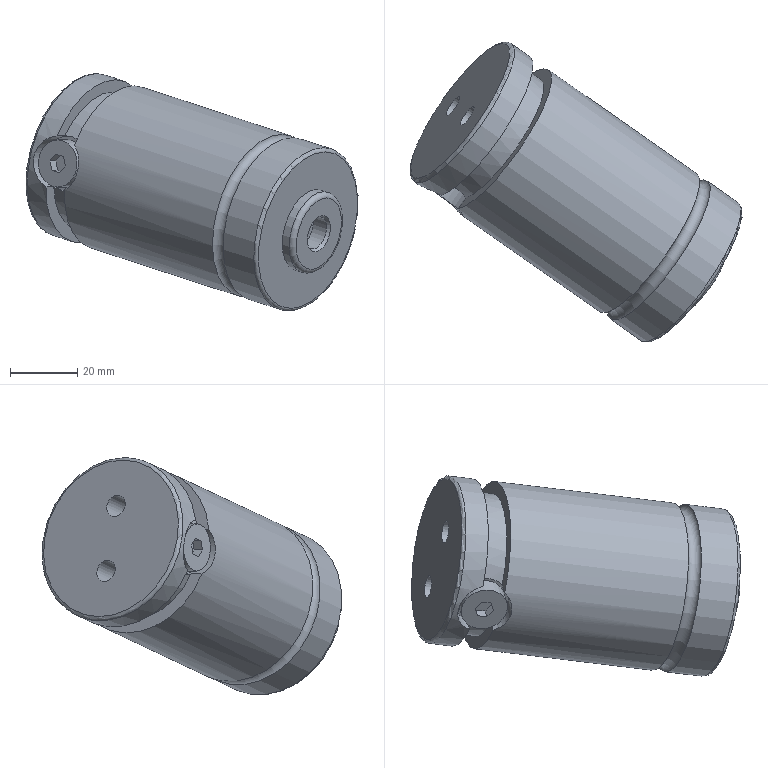Part | NX | features solid 2 | 1 solid | 38 faces | box 98.809 x 89.274 x 70.583 mm | volume 167634 mm3 | plane 17 | cylinder 13 | torus 4 | cone 4 | commonest cylinder face diameters 6.6 x3 14 x3 50.2 x3 10 x1 16.4 x1 25 x1
STEP:
#1=CARTESIAN_POINT('',(-50.295,651.708,-483.98));
#2=VERTEX_POINT('',#1);
#3=CARTESIAN_POINT('',(-55.617,655.435,-508.225));
#4=DIRECTION('',(-0.7912,0.554,0.2588));
#5=DIRECTION('',(0.212,-0.1485,0.9659));
#6=AXIS2_PLACEMENT_3D('',#3,#4,#5);
#7=CIRCLE('',#6,25.1);
#8=EDGE_CURVE('',#2,#2,#7,.T.);
#9=ORIENTED_EDGE('',*,*,#8,.F.);
#10=EDGE_LOOP('',(#9));
#11=FACE_BOUND('',#10,.T.);
#12=CARTESIAN_POINT('',(-47.13,649.492,-485.016));
#13=VERTEX_POINT('',#12);
#14=CARTESIAN_POINT('',(-52.452,653.218,-509.26));
#15=DIRECTION('',(-0.7912,0.554,0.2588));
#16=DIRECTION('',(0.212,-0.1485,0.9659));
#17=AXIS2_PLACEMENT_3D('',#14,#15,#16);
#18=CIRCLE('',#17,25.1);
#19=EDGE_CURVE('',#13,#13,#18,.T.);
#20=ORIENTED_EDGE('',*,*,#19,.T.);
#21=EDGE_LOOP('',(#20));
#22=FACE_BOUND('',#21,.T.);
#23=CARTESIAN_POINT('',(-54.034,654.327,-508.743));
#24=DIRECTION('',(0.7912,-0.554,-0.2588));
#25=DIRECTION('',(-0.5736,-0.8192,0.));
#26=AXIS2_PLACEMENT_3D('',#23,#24,#25);
#27=TOROIDAL_SURFACE('',#26,25.1,2.);
#28=ADVANCED_FACE('',(#11,#22),#27,.F.);
#29=CARTESIAN_POINT('',(-38.031,643.121,-487.992));
#30=VERTEX_POINT('',#29);
#31=CARTESIAN_POINT('',(-43.353,646.847,-512.237));
#32=DIRECTION('',(-0.7912,0.554,0.2588));
#33=DIRECTION('',(0.212,-0.1485,0.9659));
#34=AXIS2_PLACEMENT_3D('',#31,#32,#33);
#35=CIRCLE('',#34,25.1);
#36=EDGE_CURVE('',#30,#30,#35,.T.);
#37=ORIENTED_EDGE('',*,*,#36,.F.);
#38=EDGE_LOOP('',(#37));
#39=FACE_BOUND('',#38,.T.);
#40=CARTESIAN_POINT('',(-37.452,642.715,-489.217));
#41=VERTEX_POINT('',#40);
#42=CARTESIAN_POINT('',(-42.562,646.293,-512.495));
#43=DIRECTION('',(-0.7912,0.554,0.2588));
#44=DIRECTION('',(0.212,-0.1485,0.9659));
#45=AXIS2_PLACEMENT_3D('',#42,#43,#44);
#46=CIRCLE('',#45,24.1);
#47=EDGE_CURVE('',#41,#41,#46,.T.);
#48=ORIENTED_EDGE('',*,*,#47,.T.);
#49=EDGE_LOOP('',(#48));
#50=FACE_BOUND('',#49,.T.);
#51=CARTESIAN_POINT('',(-43.353,646.847,-512.237));
#52=DIRECTION('',(0.7912,-0.554,-0.2588));
#53=DIRECTION('',(-0.5736,-0.8192,0.));
#54=AXIS2_PLACEMENT_3D('',#51,#52,#53);
#55=TOROIDAL_SURFACE('',#54,24.1,1.);
#56=ADVANCED_FACE('',(#39,#50),#55,.T.);
#57=ORIENTED_EDGE('',*,*,#19,.F.);
#58=EDGE_LOOP('',(#57));
#59=FACE_BOUND('',#58,.T.);
#60=ORIENTED_EDGE('',*,*,#36,.T.);
#61=EDGE_LOOP('',(#60));
#62=FACE_BOUND('',#61,.T.);
#63=CARTESIAN_POINT('',(-47.902,650.033,-510.748));
#64=DIRECTION('',(-0.7912,0.554,0.2588));
#65=DIRECTION('',(0.5736,0.8192,0.));
#66=AXIS2_PLACEMENT_3D('',#63,#64,#65);
#67=CYLINDRICAL_SURFACE('',#66,25.1);
#68=ADVANCED_FACE('',(#59,#62),#67,.T.);
#69=CARTESIAN_POINT('',(-109.724,668.701,-487.213));
#70=VERTEX_POINT('',#69);
#71=CARTESIAN_POINT('',(-112.63,670.737,-500.456));
#72=VERTEX_POINT('',#71);
#73=CARTESIAN_POINT('',(-99.61,686.239,-493.835));
#74=DIRECTION('',(-0.7912,0.554,0.2588));
#75=DIRECTION('',(0.212,-0.1485,0.9659));
#76=AXIS2_PLACEMENT_3D('',#73,#74,#75);
#77=CIRCLE('',#76,21.3);
#78=EDGE_CURVE('',#70,#72,#77,.T.);
#79=ORIENTED_EDGE('',*,*,#78,.T.);
#80=CARTESIAN_POINT('',(-118.171,675.044,-499.566));
#81=VERTEX_POINT('',#80);
#82=CARTESIAN_POINT('',(-118.171,675.044,-499.566));
#83=CARTESIAN_POINT('',(-116.313,674.102,-500.892));
#84=CARTESIAN_POINT('',(-114.258,672.429,-501.217));
#85=CARTESIAN_POINT('',(-112.63,670.737,-500.456));
#86=B_SPLINE_CURVE_WITH_KNOTS('',3,(#82,#83,#84,#85),.UNSPECIFIED.,.F.,.F.,(4,4),(0.,0.007303),.UNSPECIFIED.);
#87=EDGE_CURVE('',#81,#72,#86,.T.);
#88=ORIENTED_EDGE('',*,*,#87,.F.);
#89=CARTESIAN_POINT('',(-114.859,672.725,-484.479));
#90=VERTEX_POINT('',#89);
#91=CARTESIAN_POINT('',(-105.149,690.117,-492.023));
#92=DIRECTION('',(-0.7912,0.554,0.2588));
#93=DIRECTION('',(0.212,-0.1485,0.9659));
#94=AXIS2_PLACEMENT_3D('',#91,#92,#93);
#95=CIRCLE('',#94,21.3);
#96=EDGE_CURVE('',#90,#81,#95,.T.);
#97=ORIENTED_EDGE('',*,*,#96,.F.);
#98=CARTESIAN_POINT('',(-109.724,668.701,-487.213));
#99=CARTESIAN_POINT('',(-110.787,669.998,-485.402));
#100=CARTESIAN_POINT('',(-112.684,671.561,-484.362));
#101=CARTESIAN_POINT('',(-114.859,672.725,-484.479));
#102=B_SPLINE_CURVE_WITH_KNOTS('',3,(#98,#99,#100,#101),.UNSPECIFIED.,.F.,.F.,(4,4),(0.,0.007305),.UNSPECIFIED.);
#103=EDGE_CURVE('',#70,#90,#102,.T.);
#104=ORIENTED_EDGE('',*,*,#103,.F.);
#105=EDGE_LOOP('',(#79,#88,#97,#104));
#106=FACE_BOUND('',#105,.T.);
#107=CARTESIAN_POINT('',(-102.379,688.178,-492.929));
#108=DIRECTION('',(-0.7912,0.554,0.2588));
#109=DIRECTION('',(0.5736,0.8192,0.));
#110=AXIS2_PLACEMENT_3D('',#107,#108,#109);
#111=CYLINDRICAL_SURFACE('',#110,21.3);
#112=ADVANCED_FACE('',(#106),#111,.T.);
#113=CARTESIAN_POINT('',(-105.366,690.269,-465.966));
#114=VERTEX_POINT('',#113);
#115=CARTESIAN_POINT('',(-110.687,693.995,-490.211));
#116=DIRECTION('',(-0.7912,0.554,0.2588));
#117=DIRECTION('',(0.212,-0.1485,0.9659));
#118=AXIS2_PLACEMENT_3D('',#115,#116,#117);
#119=CIRCLE('',#118,25.1);
#120=EDGE_CURVE('',#114,#114,#119,.T.);
#121=ORIENTED_EDGE('',*,*,#120,.F.);
#122=EDGE_LOOP('',(#121));
#123=FACE_BOUND('',#122,.T.);
#124=CARTESIAN_POINT('',(-117.175,669.417,-484.479));
#125=VERTEX_POINT('',#124);
#126=CARTESIAN_POINT('',(-120.487,671.736,-499.566));
#127=VERTEX_POINT('',#126);
#128=CARTESIAN_POINT('',(-105.149,690.117,-492.023));
#129=DIRECTION('',(-0.7912,0.554,0.2588));
#130=DIRECTION('',(0.212,-0.1485,0.9659));
#131=AXIS2_PLACEMENT_3D('',#128,#129,#130);
#132=CIRCLE('',#131,25.1);
#133=EDGE_CURVE('',#125,#127,#132,.T.);
#134=ORIENTED_EDGE('',*,*,#133,.T.);
#135=CARTESIAN_POINT('',(-117.175,669.417,-484.479));
#136=CARTESIAN_POINT('',(-118.703,670.274,-484.563));
#137=CARTESIAN_POINT('',(-121.8,671.637,-485.825));
#138=CARTESIAN_POINT('',(-124.63,672.867,-490.401));
#139=CARTESIAN_POINT('',(-124.012,673.182,-495.851));
#140=CARTESIAN_POINT('',(-121.788,672.435,-498.623));
#141=CARTESIAN_POINT('',(-120.487,671.736,-499.566));
#142=B_SPLINE_CURVE_WITH_KNOTS('',3,(#135,#136,#137,#138,#139,#140,#141),.UNSPECIFIED.,.F.,.F.,(4,1,1,1,4),(-0.01037,-0.005185,-0.000001062,0.005183,0.01037),.UNSPECIFIED.);
#143=EDGE_CURVE('',#125,#127,#142,.T.);
#144=ORIENTED_EDGE('',*,*,#143,.F.);
#145=EDGE_LOOP('',(#134,#144));
#146=FACE_BOUND('',#145,.T.);
#147=CARTESIAN_POINT('',(-107.918,692.056,-491.117));
#148=DIRECTION('',(-0.7912,0.554,0.2588));
#149=DIRECTION('',(0.5736,0.8192,0.));
#150=AXIS2_PLACEMENT_3D('',#147,#148,#149);
#151=CYLINDRICAL_SURFACE('',#150,25.1);
#152=ADVANCED_FACE('',(#123,#146),#151,.T.);
#153=CARTESIAN_POINT('',(-106.369,690.972,-466.674));
#154=VERTEX_POINT('',#153);
#155=CARTESIAN_POINT('',(-111.479,694.549,-489.952));
#156=DIRECTION('',(-0.7912,0.554,0.2588));
#157=DIRECTION('',(0.212,-0.1485,0.9659));
#158=AXIS2_PLACEMENT_3D('',#155,#156,#157);
#159=CIRCLE('',#158,24.1);
#160=EDGE_CURVE('',#154,#154,#159,.T.);
#161=ORIENTED_EDGE('',*,*,#160,.F.);
#162=EDGE_LOOP('',(#161));
#163=FACE_BOUND('',#162,.T.);
#164=ORIENTED_EDGE('',*,*,#120,.T.);
#165=EDGE_LOOP('',(#164));
#166=FACE_BOUND('',#165,.T.);
#167=CARTESIAN_POINT('',(-110.687,693.995,-490.211));
#168=DIRECTION('',(0.7912,-0.554,-0.2588));
#169=DIRECTION('',(-0.5736,-0.8192,0.));
#170=AXIS2_PLACEMENT_3D('',#167,#168,#169);
#171=TOROIDAL_SURFACE('',#170,24.1,1.);
#172=ADVANCED_FACE('',(#163,#166),#171,.T.);
#173=CARTESIAN_POINT('',(-37.854,642.997,-501.094));
#174=VERTEX_POINT('',#173);
#175=CARTESIAN_POINT('',(-40.504,644.853,-513.168));
#176=DIRECTION('',(-0.7912,0.554,0.2588));
#177=DIRECTION('',(0.212,-0.1485,0.9659));
#178=AXIS2_PLACEMENT_3D('',#175,#176,#177);
#179=CIRCLE('',#178,12.5);
#180=EDGE_CURVE('',#174,#174,#179,.T.);
#181=ORIENTED_EDGE('',*,*,#180,.F.);
#182=EDGE_LOOP('',(#181));
#183=FACE_BOUND('',#182,.T.);
#184=CARTESIAN_POINT('',(-36.985,642.389,-502.931));
#185=VERTEX_POINT('',#184);
#186=CARTESIAN_POINT('',(-39.317,644.022,-513.557));
#187=DIRECTION('',(-0.7912,0.554,0.2588));
#188=DIRECTION('',(0.212,-0.1485,0.9659));
#189=AXIS2_PLACEMENT_3D('',#186,#187,#188);
#190=CIRCLE('',#189,11.);
#191=EDGE_CURVE('',#185,#185,#190,.T.);
#192=ORIENTED_EDGE('',*,*,#191,.T.);
#193=EDGE_LOOP('',(#192));
#194=FACE_BOUND('',#193,.T.);
#195=CARTESIAN_POINT('',(-40.504,644.853,-513.168));
#196=DIRECTION('',(0.7912,-0.554,-0.2588));
#197=DIRECTION('',(-0.5736,-0.8192,0.));
#198=AXIS2_PLACEMENT_3D('',#195,#196,#197);
#199=TOROIDAL_SURFACE('',#198,11.,1.5);
#200=ADVANCED_FACE('',(#183,#194),#199,.T.);
#201=CARTESIAN_POINT('',(-39.911,644.437,-500.421));
#202=VERTEX_POINT('',#201);
#203=CARTESIAN_POINT('',(-42.562,646.293,-512.495));
#204=DIRECTION('',(0.7912,-0.554,-0.2588));
#205=DIRECTION('',(0.212,-0.1485,0.9659));
#206=AXIS2_PLACEMENT_3D('',#203,#204,#205);
#207=CIRCLE('',#206,12.5);
#208=EDGE_CURVE('',#202,#202,#207,.T.);
#209=ORIENTED_EDGE('',*,*,#208,.T.);
#210=EDGE_LOOP('',(#209));
#211=FACE_BOUND('',#210,.T.);
#212=ORIENTED_EDGE('',*,*,#180,.T.);
#213=EDGE_LOOP('',(#212));
#214=FACE_BOUND('',#213,.T.);
#215=CARTESIAN_POINT('',(-41.533,645.573,-512.832));
#216=DIRECTION('',(-0.7912,0.554,0.2588));
#217=DIRECTION('',(0.5736,0.8192,0.));
#218=AXIS2_PLACEMENT_3D('',#215,#216,#217);
#219=CYLINDRICAL_SURFACE('',#218,12.5);
#220=ADVANCED_FACE('',(#211,#214),#219,.T.);
#221=CARTESIAN_POINT('',(-100.146,686.614,-486.723));
#222=VERTEX_POINT('',#221);
#223=CARTESIAN_POINT('',(-103.354,688.86,-485.674));
#224=VERTEX_POINT('',#223);
#225=CARTESIAN_POINT('',(-101.75,687.737,-486.198));
#226=DIRECTION('',(-0.7912,0.554,0.2588));
#227=VECTOR('',#226,1000.);
#228=LINE('',#225,#227);
#229=EDGE_CURVE('',#222,#224,#228,.T.);
#230=ORIENTED_EDGE('',*,*,#229,.F.);
#231=CARTESIAN_POINT('',(-103.354,688.86,-485.674));
#232=CARTESIAN_POINT('',(-103.619,688.482,-485.674));
#233=CARTESIAN_POINT('',(-103.485,687.466,-485.647));
#234=CARTESIAN_POINT('',(-102.511,686.497,-485.862));
#235=CARTESIAN_POINT('',(-101.327,685.953,-486.352));
#236=CARTESIAN_POINT('',(-100.411,686.236,-486.723));
#237=CARTESIAN_POINT('',(-100.146,686.614,-486.723));
#238=B_SPLINE_CURVE_WITH_KNOTS('',3,(#231,#232,#233,#234,#235,#236,#237),.UNSPECIFIED.,.F.,.F.,(4,1,1,1,4),(0.,0.001359,0.002718,0.004077,0.005435),.UNSPECIFIED.);
#239=EDGE_CURVE('',#224,#222,#238,.T.);
#240=ORIENTED_EDGE('',*,*,#239,.F.);
#241=EDGE_LOOP('',(#230,#240));
#242=FACE_BOUND('',#241,.T.);
#243=CARTESIAN_POINT('',(-110.058,693.555,-483.481));
#244=VERTEX_POINT('',#243);
#245=CARTESIAN_POINT('',(-109.358,693.065,-480.293));
#246=DIRECTION('',(-0.7912,0.554,0.2588));
#247=DIRECTION('',(-0.212,0.1485,-0.9659));
#248=AXIS2_PLACEMENT_3D('',#245,#246,#247);
#249=CIRCLE('',#248,3.3);
#250=EDGE_CURVE('',#244,#244,#249,.T.);
#251=ORIENTED_EDGE('',*,*,#250,.T.);
#252=EDGE_LOOP('',(#251));
#253=FACE_BOUND('',#252,.T.);
#254=CARTESIAN_POINT('',(-96.211,683.859,-488.01));
#255=VERTEX_POINT('',#254);
#256=CARTESIAN_POINT('',(-95.512,683.369,-484.822));
#257=DIRECTION('',(0.7912,-0.554,-0.2588));
#258=DIRECTION('',(-0.212,0.1485,-0.9659));
#259=AXIS2_PLACEMENT_3D('',#256,#257,#258);
#260=CIRCLE('',#259,3.3);
#261=EDGE_CURVE('',#255,#255,#260,.T.);
#262=ORIENTED_EDGE('',*,*,#261,.T.);
#263=EDGE_LOOP('',(#262));
#264=FACE_BOUND('',#263,.T.);
#265=CARTESIAN_POINT('',(-102.435,688.217,-482.558));
#266=DIRECTION('',(0.7912,-0.554,-0.2588));
#267=DIRECTION('',(-0.5736,-0.8192,0.));
#268=AXIS2_PLACEMENT_3D('',#265,#266,#267);
#269=CYLINDRICAL_SURFACE('',#268,3.3);
#270=ADVANCED_FACE('',(#242,#253,#264),#269,.F.);
#271=ORIENTED_EDGE('',*,*,#261,.F.);
#272=EDGE_LOOP('',(#271));
#273=FACE_BOUND('',#272,.T.);
#274=CARTESIAN_POINT('',(-102.633,688.355,-482.493));
#275=VERTEX_POINT('',#274);
#276=VERTEX_LOOP('',#275);
#277=FACE_BOUND('',#276,.T.);
#278=CARTESIAN_POINT('',(-99.072,685.862,-483.658));
#279=DIRECTION('',(0.7912,-0.554,-0.2588));
#280=DIRECTION('',(-0.5736,-0.8192,0.));
#281=AXIS2_PLACEMENT_3D('',#278,#279,#280);
#282=CONICAL_SURFACE('',#281,1.65,0.3514);
#283=ADVANCED_FACE('',(#273,#277),#282,.T.);
#284=CARTESIAN_POINT('',(-106.873,691.325,-501.812));
#285=VERTEX_POINT('',#284);
#286=VERTEX_LOOP('',#285);
#287=FACE_BOUND('',#286,.T.);
#288=CARTESIAN_POINT('',(-99.052,685.848,-500.953));
#289=VERTEX_POINT('',#288);
#290=CARTESIAN_POINT('',(-99.752,686.338,-504.141));
#291=DIRECTION('',(-0.7912,0.554,0.2588));
#292=DIRECTION('',(0.212,-0.1485,0.9659));
#293=AXIS2_PLACEMENT_3D('',#290,#291,#292);
#294=CIRCLE('',#293,3.3);
#295=EDGE_CURVE('',#289,#289,#294,.T.);
#296=ORIENTED_EDGE('',*,*,#295,.T.);
#297=EDGE_LOOP('',(#296));
#298=FACE_BOUND('',#297,.T.);
#299=CARTESIAN_POINT('',(-103.313,688.831,-502.976));
#300=DIRECTION('',(0.7912,-0.554,-0.2588));
#301=DIRECTION('',(-0.5736,-0.8192,0.));
#302=AXIS2_PLACEMENT_3D('',#299,#300,#301);
#303=CONICAL_SURFACE('',#302,1.65,0.3514);
#304=ADVANCED_FACE('',(#287,#298),#303,.T.);
#305=CARTESIAN_POINT('',(-106.195,690.85,-498.617));
#306=VERTEX_POINT('',#305);
#307=CARTESIAN_POINT('',(-102.987,688.603,-499.666));
#308=VERTEX_POINT('',#307);
#309=CARTESIAN_POINT('',(-104.591,689.727,-499.142));
#310=DIRECTION('',(0.7912,-0.554,-0.2588));
#311=VECTOR('',#310,1000.);
#312=LINE('',#309,#311);
#313=EDGE_CURVE('',#306,#308,#312,.T.);
#314=ORIENTED_EDGE('',*,*,#313,.F.);
#315=CARTESIAN_POINT('',(-102.987,688.603,-499.666));
#316=CARTESIAN_POINT('',(-103.252,688.225,-499.666));
#317=CARTESIAN_POINT('',(-104.252,688.003,-499.693));
#318=CARTESIAN_POINT('',(-105.497,688.587,-499.478));
#319=CARTESIAN_POINT('',(-106.413,689.514,-498.987));
#320=CARTESIAN_POINT('',(-106.46,690.472,-498.617));
#321=CARTESIAN_POINT('',(-106.195,690.85,-498.617));
#322=B_SPLINE_CURVE_WITH_KNOTS('',3,(#315,#316,#317,#318,#319,#320,#321),.UNSPECIFIED.,.F.,.F.,(4,1,1,1,4),(0.,0.001359,0.002718,0.004077,0.005435),.UNSPECIFIED.);
#323=EDGE_CURVE('',#308,#306,#322,.T.);
#324=ORIENTED_EDGE('',*,*,#323,.F.);
#325=EDGE_LOOP('',(#314,#324));
#326=FACE_BOUND('',#325,.T.);
#327=ORIENTED_EDGE('',*,*,#295,.F.);
#328=EDGE_LOOP('',(#327));
#329=FACE_BOUND('',#328,.T.);
#330=CARTESIAN_POINT('',(-112.899,695.544,-496.424));
#331=VERTEX_POINT('',#330);
#332=CARTESIAN_POINT('',(-113.599,696.034,-499.612));
#333=DIRECTION('',(-0.7912,0.554,0.2588));
#334=DIRECTION('',(0.212,-0.1485,0.9659));
#335=AXIS2_PLACEMENT_3D('',#332,#333,#334);
#336=CIRCLE('',#335,3.3);
#337=EDGE_CURVE('',#331,#331,#336,.T.);
#338=ORIENTED_EDGE('',*,*,#337,.T.);
#339=EDGE_LOOP('',(#338));
#340=FACE_BOUND('',#339,.T.);
#341=CARTESIAN_POINT('',(-106.675,691.186,-501.876));
#342=DIRECTION('',(-0.7912,0.554,0.2588));
#343=DIRECTION('',(0.5736,0.8192,0.));
#344=AXIS2_PLACEMENT_3D('',#341,#342,#343);
#345=CYLINDRICAL_SURFACE('',#344,3.3);
#346=ADVANCED_FACE('',(#326,#329,#340),#345,.F.);
#347=CARTESIAN_POINT('',(-112.006,665.442,-487.213));
#348=VERTEX_POINT('',#347);
#349=CARTESIAN_POINT('',(-114.913,667.477,-500.456));
#350=VERTEX_POINT('',#349);
#351=CARTESIAN_POINT('',(-99.61,686.239,-493.835));
#352=DIRECTION('',(-0.7912,0.554,0.2588));
#353=DIRECTION('',(0.212,-0.1485,0.9659));
#354=AXIS2_PLACEMENT_3D('',#351,#352,#353);
#355=CIRCLE('',#354,25.1);
#356=EDGE_CURVE('',#348,#350,#355,.T.);
#357=ORIENTED_EDGE('',*,*,#356,.F.);
#358=CARTESIAN_POINT('',(-114.913,667.477,-500.456));
#359=CARTESIAN_POINT('',(-113.976,666.563,-500.029));
#360=CARTESIAN_POINT('',(-112.365,664.824,-498.559));
#361=CARTESIAN_POINT('',(-110.87,663.334,-494.883));
#362=CARTESIAN_POINT('',(-110.631,663.61,-490.663));
#363=CARTESIAN_POINT('',(-111.386,664.749,-488.229));
#364=CARTESIAN_POINT('',(-112.006,665.442,-487.213));
#365=B_SPLINE_CURVE_WITH_KNOTS('',3,(#358,#359,#360,#361,#362,#363,#364),.UNSPECIFIED.,.F.,.F.,(4,1,1,1,4),(-0.008143,-0.004072,-0.000000126,0.004071,0.008143),.UNSPECIFIED.);
#366=EDGE_CURVE('',#350,#348,#365,.T.);
#367=ORIENTED_EDGE('',*,*,#366,.F.);
#368=EDGE_LOOP('',(#357,#367));
#369=FACE_BOUND('',#368,.T.);
#370=ORIENTED_EDGE('',*,*,#8,.T.);
#371=EDGE_LOOP('',(#370));
#372=FACE_BOUND('',#371,.T.);
#373=CARTESIAN_POINT('',(-77.613,670.837,-501.03));
#374=DIRECTION('',(-0.7912,0.554,0.2588));
#375=DIRECTION('',(0.5736,0.8192,0.));
#376=AXIS2_PLACEMENT_3D('',#373,#374,#375);
#377=CYLINDRICAL_SURFACE('',#376,25.1);
#378=ADVANCED_FACE('',(#369,#372),#377,.T.);
#379=CARTESIAN_POINT('',(-112.387,671.869,-484.749));
#380=VERTEX_POINT('',#379);
#381=CARTESIAN_POINT('',(-114.126,673.086,-492.67));
#382=DIRECTION('',(0.5736,0.8192,0.));
#383=DIRECTION('',(0.212,-0.1485,0.9659));
#384=AXIS2_PLACEMENT_3D('',#381,#382,#383);
#385=CIRCLE('',#384,8.2);
#386=EDGE_CURVE('',#380,#380,#385,.T.);
#387=ORIENTED_EDGE('',*,*,#386,.T.);
#388=EDGE_LOOP('',(#387));
#389=FACE_BOUND('',#388,.T.);
#390=ORIENTED_EDGE('',*,*,#103,.T.);
#391=CARTESIAN_POINT('',(-116.169,670.854,-484.479));
#392=DIRECTION('',(-0.5736,-0.8192,0.));
#393=VECTOR('',#392,1000.);
#394=LINE('',#391,#393);
#395=EDGE_CURVE('',#90,#125,#394,.T.);
#396=ORIENTED_EDGE('',*,*,#395,.T.);
#397=ORIENTED_EDGE('',*,*,#143,.T.);
#398=CARTESIAN_POINT('',(-119.48,673.173,-499.566));
#399=DIRECTION('',(0.5736,0.8192,0.));
#400=VECTOR('',#399,1000.);
#401=LINE('',#398,#400);
#402=EDGE_CURVE('',#127,#81,#401,.T.);
#403=ORIENTED_EDGE('',*,*,#402,.T.);
#404=ORIENTED_EDGE('',*,*,#87,.T.);
#405=CARTESIAN_POINT('',(-113.739,669.153,-500.456));
#406=DIRECTION('',(-0.5736,-0.8192,0.));
#407=VECTOR('',#406,1000.);
#408=LINE('',#405,#407);
#409=EDGE_CURVE('',#72,#350,#408,.T.);
#410=ORIENTED_EDGE('',*,*,#409,.T.);
#411=ORIENTED_EDGE('',*,*,#366,.T.);
#412=CARTESIAN_POINT('',(-110.833,667.118,-487.213));
#413=DIRECTION('',(0.5736,0.8192,0.));
#414=VECTOR('',#413,1000.);
#415=LINE('',#412,#414);
#416=EDGE_CURVE('',#348,#70,#415,.T.);
#417=ORIENTED_EDGE('',*,*,#416,.T.);
#418=EDGE_LOOP('',(#390,#396,#397,#403,#404,#410,#411,#417));
#419=FACE_BOUND('',#418,.T.);
#420=CARTESIAN_POINT('',(-117.567,668.171,-492.67));
#421=DIRECTION('',(-0.5736,-0.8192,0.));
#422=DIRECTION('',(0.212,-0.1485,0.9659));
#423=AXIS2_PLACEMENT_3D('',#420,#421,#422);
#424=CYLINDRICAL_SURFACE('',#423,8.2);
#425=ADVANCED_FACE('',(#389,#419),#424,.F.);
#426=CARTESIAN_POINT('',(-112.642,672.047,-485.908));
#427=VERTEX_POINT('',#426);
#428=CARTESIAN_POINT('',(-114.126,673.086,-492.67));
#429=DIRECTION('',(-0.5736,-0.8192,0.));
#430=DIRECTION('',(0.212,-0.1485,0.9659));
#431=AXIS2_PLACEMENT_3D('',#428,#429,#430);
#432=CIRCLE('',#431,7.);
#433=EDGE_CURVE('',#427,#427,#432,.T.);
#434=ORIENTED_EDGE('',*,*,#433,.T.);
#435=EDGE_LOOP('',(#434));
#436=FACE_BOUND('',#435,.T.);
#437=CARTESIAN_POINT('',(-115.51,667.951,-485.908));
#438=VERTEX_POINT('',#437);
#439=CARTESIAN_POINT('',(-116.994,668.99,-492.67));
#440=DIRECTION('',(-0.5736,-0.8192,0.));
#441=DIRECTION('',(0.212,-0.1485,0.9659));
#442=AXIS2_PLACEMENT_3D('',#439,#440,#441);
#443=CIRCLE('',#442,7.);
#444=EDGE_CURVE('',#438,#438,#443,.T.);
#445=ORIENTED_EDGE('',*,*,#444,.F.);
#446=EDGE_LOOP('',(#445));
#447=FACE_BOUND('',#446,.T.);
#448=CARTESIAN_POINT('',(-103.17,688.732,-492.67));
#449=DIRECTION('',(0.5736,0.8192,0.));
#450=DIRECTION('',(-0.212,0.1485,-0.9659));
#451=AXIS2_PLACEMENT_3D('',#448,#449,#450);
#452=CYLINDRICAL_SURFACE('',#451,7.);
#453=ADVANCED_FACE('',(#436,#447),#452,.T.);
#454=CARTESIAN_POINT('',(-103.17,688.732,-492.67));
#455=DIRECTION('',(0.5736,0.8192,0.));
#456=DIRECTION('',(0.212,-0.1485,0.9659));
#457=AXIS2_PLACEMENT_3D('',#454,#455,#456);
#458=CIRCLE('',#457,7.);
#459=EDGE_CURVE('',#308,#306,#458,.T.);
#460=ORIENTED_EDGE('',*,*,#459,.F.);
#461=ORIENTED_EDGE('',*,*,#323,.T.);
#462=EDGE_LOOP('',(#460,#461));
#463=FACE_BOUND('',#462,.T.);
#464=CARTESIAN_POINT('',(-103.17,688.732,-492.67));
#465=DIRECTION('',(0.5736,0.8192,0.));
#466=DIRECTION('',(-0.212,0.1485,-0.9659));
#467=AXIS2_PLACEMENT_3D('',#464,#465,#466);
#468=CYLINDRICAL_SURFACE('',#467,7.);
#469=ADVANCED_FACE('',(#463),#468,.T.);
#470=ORIENTED_EDGE('',*,*,#239,.T.);
#471=CARTESIAN_POINT('',(-103.17,688.732,-492.67));
#472=DIRECTION('',(0.5736,0.8192,0.));
#473=DIRECTION('',(0.212,-0.1485,0.9659));
#474=AXIS2_PLACEMENT_3D('',#471,#472,#473);
#475=CIRCLE('',#474,7.);
#476=EDGE_CURVE('',#224,#222,#475,.T.);
#477=ORIENTED_EDGE('',*,*,#476,.F.);
#478=EDGE_LOOP('',(#470,#477));
#479=FACE_BOUND('',#478,.T.);
#480=CARTESIAN_POINT('',(-103.17,688.732,-492.67));
#481=DIRECTION('',(0.5736,0.8192,0.));
#482=DIRECTION('',(-0.212,0.1485,-0.9659));
#483=AXIS2_PLACEMENT_3D('',#480,#481,#482);
#484=CYLINDRICAL_SURFACE('',#483,7.);
#485=ADVANCED_FACE('',(#479),#484,.T.);
#486=CARTESIAN_POINT('',(-36.105,648.609,-513.557));
#487=VERTEX_POINT('',#486);
#488=CARTESIAN_POINT('',(-39.317,644.022,-513.557));
#489=DIRECTION('',(0.7912,-0.554,-0.2588));
#490=DIRECTION('',(0.5736,0.8192,0.));
#491=AXIS2_PLACEMENT_3D('',#488,#489,#490);
#492=CIRCLE('',#491,5.6);
#493=EDGE_CURVE('',#487,#487,#492,.T.);
#494=ORIENTED_EDGE('',*,*,#493,.T.);
#495=EDGE_LOOP('',(#494));
#496=FACE_BOUND('',#495,.T.);
#497=CARTESIAN_POINT('',(-37.241,648.671,-513.298));
#498=VERTEX_POINT('',#497);
#499=CARTESIAN_POINT('',(-40.109,644.576,-513.298));
#500=DIRECTION('',(-0.7912,0.554,0.2588));
#501=DIRECTION('',(0.5736,0.8192,0.));
#502=AXIS2_PLACEMENT_3D('',#499,#500,#501);
#503=CIRCLE('',#502,5.);
#504=EDGE_CURVE('',#498,#498,#503,.T.);
#505=ORIENTED_EDGE('',*,*,#504,.T.);
#506=EDGE_LOOP('',(#505));
#507=FACE_BOUND('',#506,.T.);
#508=CARTESIAN_POINT('',(-39.713,644.299,-513.427));
#509=DIRECTION('',(0.7912,-0.554,-0.2588));
#510=DIRECTION('',(-0.5736,-0.8192,0.));
#511=AXIS2_PLACEMENT_3D('',#508,#509,#510);
#512=CONICAL_SURFACE('',#511,5.3,0.5404);
#513=ADVANCED_FACE('',(#496,#507),#512,.F.);
#514=ORIENTED_EDGE('',*,*,#504,.F.);
#515=EDGE_LOOP('',(#514));
#516=FACE_BOUND('',#515,.T.);
#517=CARTESIAN_POINT('',(-41.197,651.441,-512.004));
#518=VERTEX_POINT('',#517);
#519=CARTESIAN_POINT('',(-44.065,647.346,-512.004));
#520=DIRECTION('',(-0.7912,0.554,0.2588));
#521=DIRECTION('',(0.5736,0.8192,0.));
#522=AXIS2_PLACEMENT_3D('',#519,#520,#521);
#523=CIRCLE('',#522,5.);
#524=EDGE_CURVE('',#518,#518,#523,.T.);
#525=ORIENTED_EDGE('',*,*,#524,.T.);
#526=EDGE_LOOP('',(#525));
#527=FACE_BOUND('',#526,.T.);
#528=CARTESIAN_POINT('',(-42.087,645.961,-512.651));
#529=DIRECTION('',(-0.7912,0.554,0.2588));
#530=DIRECTION('',(0.5736,0.8192,0.));
#531=AXIS2_PLACEMENT_3D('',#528,#529,#530);
#532=CYLINDRICAL_SURFACE('',#531,5.);
#533=ADVANCED_FACE('',(#516,#527),#532,.F.);
#534=CARTESIAN_POINT('',(-42.172,650.049,-512.004));
#535=VERTEX_POINT('',#534);
#536=CARTESIAN_POINT('',(-44.065,647.346,-512.004));
#537=DIRECTION('',(-0.7912,0.554,0.2588));
#538=DIRECTION('',(0.5736,0.8192,0.));
#539=AXIS2_PLACEMENT_3D('',#536,#537,#538);
#540=CIRCLE('',#539,3.3);
#541=EDGE_CURVE('',#535,#535,#540,.T.);
#542=ORIENTED_EDGE('',*,*,#541,.F.);
#543=EDGE_LOOP('',(#542));
#544=FACE_BOUND('',#543,.T.);
#545=CARTESIAN_POINT('',(-48.502,654.481,-509.933));
#546=VERTEX_POINT('',#545);
#547=CARTESIAN_POINT('',(-50.395,651.778,-509.933));
#548=DIRECTION('',(-0.7912,0.554,0.2588));
#549=DIRECTION('',(0.5736,0.8192,0.));
#550=AXIS2_PLACEMENT_3D('',#547,#548,#549);
#551=CIRCLE('',#550,3.3);
#552=EDGE_CURVE('',#546,#546,#551,.T.);
#553=ORIENTED_EDGE('',*,*,#552,.T.);
#554=EDGE_LOOP('',(#553));
#555=FACE_BOUND('',#554,.T.);
#556=CARTESIAN_POINT('',(-47.23,649.562,-510.968));
#557=DIRECTION('',(-0.7912,0.554,0.2588));
#558=DIRECTION('',(0.5736,0.8192,0.));
#559=AXIS2_PLACEMENT_3D('',#556,#557,#558);
#560=CYLINDRICAL_SURFACE('',#559,3.3);
#561=ADVANCED_FACE('',(#544,#555),#560,.F.);
#562=CARTESIAN_POINT('',(-51.977,652.886,-509.416));
#563=VERTEX_POINT('',#562);
#564=VERTEX_LOOP('',#563);
#565=FACE_BOUND('',#564,.T.);
#566=ORIENTED_EDGE('',*,*,#552,.F.);
#567=EDGE_LOOP('',(#566));
#568=FACE_BOUND('',#567,.T.);
#569=CARTESIAN_POINT('',(-51.186,652.332,-509.674));
#570=DIRECTION('',(0.7912,-0.554,-0.2588));
#571=DIRECTION('',(-0.5736,-0.8192,0.));
#572=AXIS2_PLACEMENT_3D('',#569,#570,#571);
#573=CONICAL_SURFACE('',#572,1.65,1.026);
#574=ADVANCED_FACE('',(#565,#568),#573,.F.);
#575=ORIENTED_EDGE('',*,*,#524,.F.);
#576=EDGE_LOOP('',(#575));
#577=FACE_BOUND('',#576,.T.);
#578=ORIENTED_EDGE('',*,*,#541,.T.);
#579=EDGE_LOOP('',(#578));
#580=FACE_BOUND('',#579,.T.);
#581=CARTESIAN_POINT('',(-41.685,650.745,-512.004));
#582=DIRECTION('',(-0.7912,0.554,0.2588));
#583=DIRECTION('',(0.5736,0.8192,0.));
#584=AXIS2_PLACEMENT_3D('',#581,#582,#583);
#585=PLANE('',#584);
#586=ADVANCED_FACE('',(#577,#580),#585,.F.);
#587=CARTESIAN_POINT('',(-114.71,667.391,-493.417));
#588=VERTEX_POINT('',#587);
#589=CARTESIAN_POINT('',(-115.322,667.82,-490.629));
#590=VERTEX_POINT('',#589);
#591=CARTESIAN_POINT('',(-115.725,668.102,-488.79));
#592=DIRECTION('',(-0.212,0.1485,0.9659));
#593=VECTOR('',#592,1000.);
#594=LINE('',#591,#593);
#595=EDGE_CURVE('',#588,#590,#594,.T.);
#596=ORIENTED_EDGE('',*,*,#595,.T.);
#597=CARTESIAN_POINT('',(-113.601,670.277,-490.629));
#598=VERTEX_POINT('',#597);
#599=CARTESIAN_POINT('',(-115.895,667.,-490.629));
#600=DIRECTION('',(0.5736,0.8192,0.));
#601=VECTOR('',#600,1000.);
#602=LINE('',#599,#601);
#603=EDGE_CURVE('',#590,#598,#602,.T.);
#604=ORIENTED_EDGE('',*,*,#603,.T.);
#605=CARTESIAN_POINT('',(-112.989,669.848,-493.417));
#606=VERTEX_POINT('',#605);
#607=CARTESIAN_POINT('',(-113.601,670.277,-490.629));
#608=DIRECTION('',(0.212,-0.1485,-0.9659));
#609=VECTOR('',#608,1000.);
#610=LINE('',#607,#609);
#611=EDGE_CURVE('',#598,#606,#610,.T.);
#612=ORIENTED_EDGE('',*,*,#611,.T.);
#613=CARTESIAN_POINT('',(-115.283,666.572,-493.417));
#614=DIRECTION('',(0.5736,0.8192,0.));
#615=VECTOR('',#614,1000.);
#616=LINE('',#613,#615);
#617=EDGE_CURVE('',#588,#606,#616,.T.);
#618=ORIENTED_EDGE('',*,*,#617,.F.);
#619=EDGE_LOOP('',(#596,#604,#612,#618));
#620=FACE_BOUND('',#619,.T.);
#621=CARTESIAN_POINT('',(-115.895,667.,-490.629));
#622=DIRECTION('',(0.7912,-0.554,0.2588));
#623=DIRECTION('',(0.212,-0.1485,-0.9659));
#624=AXIS2_PLACEMENT_3D('',#621,#622,#623);
#625=PLANE('',#624);
#626=ADVANCED_FACE('',(#620),#625,.F.);
#627=CARTESIAN_POINT('',(-117.606,669.419,-489.882));
#628=VERTEX_POINT('',#627);
#629=CARTESIAN_POINT('',(-121.189,671.928,-488.71));
#630=DIRECTION('',(-0.7912,0.554,0.2588));
#631=VECTOR('',#630,1000.);
#632=LINE('',#629,#631);
#633=EDGE_CURVE('',#590,#628,#632,.T.);
#634=ORIENTED_EDGE('',*,*,#633,.T.);
#635=CARTESIAN_POINT('',(-115.885,671.876,-489.882));
#636=VERTEX_POINT('',#635);
#637=CARTESIAN_POINT('',(-118.179,668.6,-489.882));
#638=DIRECTION('',(0.5736,0.8192,0.));
#639=VECTOR('',#638,1000.);
#640=LINE('',#637,#639);
#641=EDGE_CURVE('',#628,#636,#640,.T.);
#642=ORIENTED_EDGE('',*,*,#641,.T.);
#643=CARTESIAN_POINT('',(-115.885,671.876,-489.882));
#644=DIRECTION('',(0.7912,-0.554,-0.2588));
#645=VECTOR('',#644,1000.);
#646=LINE('',#643,#645);
#647=EDGE_CURVE('',#636,#598,#646,.T.);
#648=ORIENTED_EDGE('',*,*,#647,.T.);
#649=ORIENTED_EDGE('',*,*,#603,.F.);
#650=EDGE_LOOP('',(#634,#642,#648,#649));
#651=FACE_BOUND('',#650,.T.);
#652=CARTESIAN_POINT('',(-118.179,668.6,-489.882));
#653=DIRECTION('',(0.212,-0.1485,0.9659));
#654=DIRECTION('',(0.5736,0.8192,0.));
#655=AXIS2_PLACEMENT_3D('',#652,#653,#654);
#656=PLANE('',#655);
#657=ADVANCED_FACE('',(#651),#656,.F.);
#658=CARTESIAN_POINT('',(-119.278,670.59,-491.923));
#659=VERTEX_POINT('',#658);
#660=CARTESIAN_POINT('',(-120.38,671.362,-493.269));
#661=DIRECTION('',(-0.5792,0.4056,-0.7071));
#662=VECTOR('',#661,1000.);
#663=LINE('',#660,#662);
#664=EDGE_CURVE('',#628,#659,#663,.T.);
#665=ORIENTED_EDGE('',*,*,#664,.T.);
#666=CARTESIAN_POINT('',(-117.557,673.047,-491.923));
#667=VERTEX_POINT('',#666);
#668=CARTESIAN_POINT('',(-119.851,669.771,-491.923));
#669=DIRECTION('',(0.5736,0.8192,0.));
#670=VECTOR('',#669,1000.);
#671=LINE('',#668,#670);
#672=EDGE_CURVE('',#659,#667,#671,.T.);
#673=ORIENTED_EDGE('',*,*,#672,.T.);
#674=CARTESIAN_POINT('',(-117.557,673.047,-491.923));
#675=DIRECTION('',(0.5792,-0.4056,0.7071));
#676=VECTOR('',#675,1000.);
#677=LINE('',#674,#676);
#678=EDGE_CURVE('',#667,#636,#677,.T.);
#679=ORIENTED_EDGE('',*,*,#678,.T.);
#680=ORIENTED_EDGE('',*,*,#641,.F.);
#681=EDGE_LOOP('',(#665,#673,#679,#680));
#682=FACE_BOUND('',#681,.T.);
#683=CARTESIAN_POINT('',(-119.851,669.771,-491.923));
#684=DIRECTION('',(-0.5792,0.4056,0.7071));
#685=DIRECTION('',(0.5792,-0.4056,0.7071));
#686=AXIS2_PLACEMENT_3D('',#683,#684,#685);
#687=PLANE('',#686);
#688=ADVANCED_FACE('',(#682),#687,.F.);
#689=CARTESIAN_POINT('',(-118.666,670.161,-494.711));
#690=VERTEX_POINT('',#689);
#691=CARTESIAN_POINT('',(-119.375,670.658,-491.479));
#692=DIRECTION('',(0.212,-0.1485,-0.9659));
#693=VECTOR('',#692,1000.);
#694=LINE('',#691,#693);
#695=EDGE_CURVE('',#659,#690,#694,.T.);
#696=ORIENTED_EDGE('',*,*,#695,.T.);
#697=CARTESIAN_POINT('',(-116.945,672.619,-494.711));
#698=VERTEX_POINT('',#697);
#699=CARTESIAN_POINT('',(-119.239,669.342,-494.711));
#700=DIRECTION('',(0.5736,0.8192,0.));
#701=VECTOR('',#700,1000.);
#702=LINE('',#699,#701);
#703=EDGE_CURVE('',#690,#698,#702,.T.);
#704=ORIENTED_EDGE('',*,*,#703,.T.);
#705=CARTESIAN_POINT('',(-116.945,672.619,-494.711));
#706=DIRECTION('',(-0.212,0.1485,0.9659));
#707=VECTOR('',#706,1000.);
#708=LINE('',#705,#707);
#709=EDGE_CURVE('',#698,#667,#708,.T.);
#710=ORIENTED_EDGE('',*,*,#709,.T.);
#711=ORIENTED_EDGE('',*,*,#672,.F.);
#712=EDGE_LOOP('',(#696,#704,#710,#711));
#713=FACE_BOUND('',#712,.T.);
#714=CARTESIAN_POINT('',(-119.239,669.342,-494.711));
#715=DIRECTION('',(-0.7912,0.554,-0.2588));
#716=DIRECTION('',(-0.212,0.1485,0.9659));
#717=AXIS2_PLACEMENT_3D('',#714,#715,#716);
#718=PLANE('',#717);
#719=ADVANCED_FACE('',(#713),#718,.F.);
#720=CARTESIAN_POINT('',(-116.382,668.562,-495.458));
#721=VERTEX_POINT('',#720);
#722=CARTESIAN_POINT('',(-116.648,668.748,-495.784));
#723=DIRECTION('',(0.5792,-0.4056,0.7071));
#724=VECTOR('',#723,1000.);
#725=LINE('',#722,#724);
#726=EDGE_CURVE('',#721,#588,#725,.T.);
#727=ORIENTED_EDGE('',*,*,#726,.T.);
#728=ORIENTED_EDGE('',*,*,#617,.T.);
#729=CARTESIAN_POINT('',(-114.661,671.019,-495.458));
#730=VERTEX_POINT('',#729);
#731=CARTESIAN_POINT('',(-112.989,669.848,-493.417));
#732=DIRECTION('',(-0.5792,0.4056,-0.7071));
#733=VECTOR('',#732,1000.);
#734=LINE('',#731,#733);
#735=EDGE_CURVE('',#606,#730,#734,.T.);
#736=ORIENTED_EDGE('',*,*,#735,.T.);
#737=CARTESIAN_POINT('',(-116.955,667.743,-495.458));
#738=DIRECTION('',(0.5736,0.8192,0.));
#739=VECTOR('',#738,1000.);
#740=LINE('',#737,#739);
#741=EDGE_CURVE('',#721,#730,#740,.T.);
#742=ORIENTED_EDGE('',*,*,#741,.F.);
#743=EDGE_LOOP('',(#727,#728,#736,#742));
#744=FACE_BOUND('',#743,.T.);
#745=CARTESIAN_POINT('',(-115.283,666.572,-493.417));
#746=DIRECTION('',(0.5792,-0.4056,-0.7071));
#747=DIRECTION('',(-0.5792,0.4056,-0.7071));
#748=AXIS2_PLACEMENT_3D('',#745,#746,#747);
#749=PLANE('',#748);
#750=ADVANCED_FACE('',(#744),#749,.F.);
#751=CARTESIAN_POINT('',(-121.107,671.87,-493.913));
#752=DIRECTION('',(0.7912,-0.554,-0.2588));
#753=VECTOR('',#752,1000.);
#754=LINE('',#751,#753);
#755=EDGE_CURVE('',#690,#721,#754,.T.);
#756=ORIENTED_EDGE('',*,*,#755,.T.);
#757=ORIENTED_EDGE('',*,*,#741,.T.);
#758=CARTESIAN_POINT('',(-114.661,671.019,-495.458));
#759=DIRECTION('',(-0.7912,0.554,0.2588));
#760=VECTOR('',#759,1000.);
#761=LINE('',#758,#760);
#762=EDGE_CURVE('',#730,#698,#761,.T.);
#763=ORIENTED_EDGE('',*,*,#762,.T.);
#764=ORIENTED_EDGE('',*,*,#703,.F.);
#765=EDGE_LOOP('',(#756,#757,#763,#764));
#766=FACE_BOUND('',#765,.T.);
#767=CARTESIAN_POINT('',(-116.955,667.743,-495.458));
#768=DIRECTION('',(-0.212,0.1485,-0.9659));
#769=DIRECTION('',(-0.5736,-0.8192,0.));
#770=AXIS2_PLACEMENT_3D('',#767,#768,#769);
#771=PLANE('',#770);
#772=ADVANCED_FACE('',(#766),#771,.F.);
#773=ORIENTED_EDGE('',*,*,#709,.F.);
#774=ORIENTED_EDGE('',*,*,#762,.F.);
#775=ORIENTED_EDGE('',*,*,#735,.F.);
#776=ORIENTED_EDGE('',*,*,#611,.F.);
#777=ORIENTED_EDGE('',*,*,#647,.F.);
#778=ORIENTED_EDGE('',*,*,#678,.F.);
#779=EDGE_LOOP('',(#773,#774,#775,#776,#777,#778));
#780=FACE_BOUND('',#779,.T.);
#781=CARTESIAN_POINT('',(-123.581,677.265,-489.952));
#782=DIRECTION('',(-0.5736,-0.8192,0.));
#783=DIRECTION('',(0.212,-0.1485,0.9659));
#784=AXIS2_PLACEMENT_3D('',#781,#782,#783);
#785=PLANE('',#784);
#786=ADVANCED_FACE('',(#780),#785,.T.);
#787=ORIENTED_EDGE('',*,*,#229,.T.);
#788=ORIENTED_EDGE('',*,*,#476,.T.);
#789=EDGE_LOOP('',(#787,#788));
#790=FACE_BOUND('',#789,.T.);
#791=CARTESIAN_POINT('',(-111.479,694.549,-489.952));
#792=DIRECTION('',(-0.5736,-0.8192,0.));
#793=DIRECTION('',(0.212,-0.1485,0.9659));
#794=AXIS2_PLACEMENT_3D('',#791,#792,#793);
#795=PLANE('',#794);
#796=ADVANCED_FACE('',(#790),#795,.F.);
#797=ORIENTED_EDGE('',*,*,#695,.F.);
#798=ORIENTED_EDGE('',*,*,#664,.F.);
#799=ORIENTED_EDGE('',*,*,#633,.F.);
#800=ORIENTED_EDGE('',*,*,#595,.F.);
#801=ORIENTED_EDGE('',*,*,#726,.F.);
#802=ORIENTED_EDGE('',*,*,#755,.F.);
#803=EDGE_LOOP('',(#797,#798,#799,#800,#801,#802));
#804=FACE_BOUND('',#803,.T.);
#805=ORIENTED_EDGE('',*,*,#444,.T.);
#806=EDGE_LOOP('',(#805));
#807=FACE_BOUND('',#806,.T.);
#808=CARTESIAN_POINT('',(-125.302,674.808,-489.952));
#809=DIRECTION('',(-0.5736,-0.8192,0.));
#810=DIRECTION('',(0.212,-0.1485,0.9659));
#811=AXIS2_PLACEMENT_3D('',#808,#809,#810);
#812=PLANE('',#811);
#813=ADVANCED_FACE('',(#804,#807),#812,.T.);
#814=ORIENTED_EDGE('',*,*,#313,.T.);
#815=ORIENTED_EDGE('',*,*,#459,.T.);
#816=EDGE_LOOP('',(#814,#815));
#817=FACE_BOUND('',#816,.T.);
#818=CARTESIAN_POINT('',(-111.479,694.549,-489.952));
#819=DIRECTION('',(-0.5736,-0.8192,0.));
#820=DIRECTION('',(0.212,-0.1485,0.9659));
#821=AXIS2_PLACEMENT_3D('',#818,#819,#820);
#822=PLANE('',#821);
#823=ADVANCED_FACE('',(#817),#822,.F.);
#824=ORIENTED_EDGE('',*,*,#433,.F.);
#825=EDGE_LOOP('',(#824));
#826=FACE_BOUND('',#825,.T.);
#827=ORIENTED_EDGE('',*,*,#386,.F.);
#828=EDGE_LOOP('',(#827));
#829=FACE_BOUND('',#828,.T.);
#830=CARTESIAN_POINT('',(-122.434,678.903,-489.952));
#831=DIRECTION('',(-0.5736,-0.8192,0.));
#832=DIRECTION('',(0.212,-0.1485,0.9659));
#833=AXIS2_PLACEMENT_3D('',#830,#831,#832);
#834=PLANE('',#833);
#835=ADVANCED_FACE('',(#826,#829),#834,.T.);
#836=ORIENTED_EDGE('',*,*,#493,.F.);
#837=EDGE_LOOP('',(#836));
#838=FACE_BOUND('',#837,.T.);
#839=ORIENTED_EDGE('',*,*,#191,.F.);
#840=EDGE_LOOP('',(#839));
#841=FACE_BOUND('',#840,.T.);
#842=CARTESIAN_POINT('',(-38.151,643.205,-508.244));
#843=DIRECTION('',(0.7912,-0.554,-0.2588));
#844=DIRECTION('',(-0.5736,-0.8192,0.));
#845=AXIS2_PLACEMENT_3D('',#842,#843,#844);
#846=PLANE('',#845);
#847=ADVANCED_FACE('',(#838,#841),#846,.T.);
#848=ORIENTED_EDGE('',*,*,#337,.F.);
#849=EDGE_LOOP('',(#848));
#850=FACE_BOUND('',#849,.T.);
#851=ORIENTED_EDGE('',*,*,#250,.F.);
#852=EDGE_LOOP('',(#851));
#853=FACE_BOUND('',#852,.T.);
#854=ORIENTED_EDGE('',*,*,#160,.T.);
#855=EDGE_LOOP('',(#854));
#856=FACE_BOUND('',#855,.T.);
#857=CARTESIAN_POINT('',(-108.924,692.76,-478.313));
#858=DIRECTION('',(-0.7912,0.554,0.2588));
#859=DIRECTION('',(0.212,-0.1485,0.9659));
#860=AXIS2_PLACEMENT_3D('',#857,#858,#859);
#861=PLANE('',#860);
#862=ADVANCED_FACE('',(#850,#853,#856),#861,.T.);
#863=ORIENTED_EDGE('',*,*,#402,.F.);
#864=ORIENTED_EDGE('',*,*,#133,.F.);
#865=ORIENTED_EDGE('',*,*,#395,.F.);
#866=ORIENTED_EDGE('',*,*,#96,.T.);
#867=EDGE_LOOP('',(#863,#864,#865,#866));
#868=FACE_BOUND('',#867,.T.);
#869=CARTESIAN_POINT('',(-100.23,686.673,-469.613));
#870=DIRECTION('',(0.7912,-0.554,-0.2588));
#871=DIRECTION('',(-0.5736,-0.8192,0.));
#872=AXIS2_PLACEMENT_3D('',#869,#870,#871);
#873=PLANE('',#872);
#874=ADVANCED_FACE('',(#868),#873,.T.);
#875=ORIENTED_EDGE('',*,*,#409,.F.);
#876=ORIENTED_EDGE('',*,*,#78,.F.);
#877=ORIENTED_EDGE('',*,*,#416,.F.);
#878=ORIENTED_EDGE('',*,*,#356,.T.);
#879=EDGE_LOOP('',(#875,#876,#877,#878));
#880=FACE_BOUND('',#879,.T.);
#881=CARTESIAN_POINT('',(-94.691,682.795,-471.425));
#882=DIRECTION('',(-0.7912,0.554,0.2588));
#883=DIRECTION('',(0.5736,0.8192,0.));
#884=AXIS2_PLACEMENT_3D('',#881,#882,#883);
#885=PLANE('',#884);
#886=ADVANCED_FACE('',(#880),#885,.T.);
#887=ORIENTED_EDGE('',*,*,#208,.F.);
#888=EDGE_LOOP('',(#887));
#889=FACE_BOUND('',#888,.T.);
#890=ORIENTED_EDGE('',*,*,#47,.F.);
#891=EDGE_LOOP('',(#890));
#892=FACE_BOUND('',#891,.T.);
#893=CARTESIAN_POINT('',(-40.007,644.504,-500.856));
#894=DIRECTION('',(0.7912,-0.554,-0.2588));
#895=DIRECTION('',(-0.5736,-0.8192,0.));
#896=AXIS2_PLACEMENT_3D('',#893,#894,#895);
#897=PLANE('',#896);
#898=ADVANCED_FACE('',(#889,#892),#897,.T.);
#899=CLOSED_SHELL('',(#28,#56,#68,#112,#152,#172,#200,#220,#270,#283,#304,#346,#378,#425,#453,#469,#485,#513,#533,#561,#574,#586,#626,#657,#688,#719,#750,#772,#786,#796,#813,#823,#835,#847,#862,#874,#886,#898));
#900=MANIFOLD_SOLID_BREP('',#899);
#901=(LENGTH_UNIT()NAMED_UNIT(*)SI_UNIT(.MILLI.,.METRE.));
#902=UNCERTAINTY_MEASURE_WITH_UNIT(LENGTH_MEASURE(0.0508),#901,'','');
#903=(NAMED_UNIT(*)PLANE_ANGLE_UNIT()SI_UNIT($,.RADIAN.));
#904=(NAMED_UNIT(*)SI_UNIT($,.STERADIAN.)SOLID_ANGLE_UNIT());
#905=(GEOMETRIC_REPRESENTATION_CONTEXT(3)GLOBAL_UNCERTAINTY_ASSIGNED_CONTEXT((#902))GLOBAL_UNIT_ASSIGNED_CONTEXT((#901,#903,#904))REPRESENTATION_CONTEXT('',''));
#906=ADVANCED_BREP_SHAPE_REPRESENTATION('',(#900),#905);